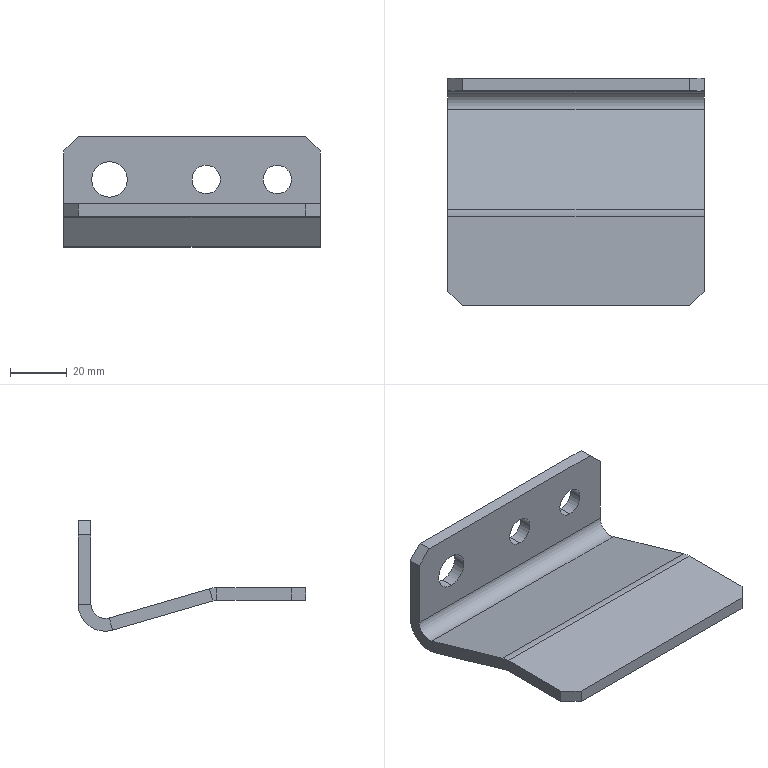Part | SolidWorks | features Chamfer 1, FlatPattern 1, ICE 1, SMBaseFlange 1, SheetMetal 1 | 1 solid | 32 faces | box 90 x 80 x 38.833 mm | volume 44176 mm3 | plane 22 | cylinder 10 | commonest cylinder face diameters 10 x6 12.5 x2 19 x2
STEP:
#1=CARTESIAN_POINT('',(75.,-4.5,-10.));
#2=VERTEX_POINT('',#1);
#3=CARTESIAN_POINT('',(75.,-4.5,-20.));
#4=VERTEX_POINT('',#3);
#5=CARTESIAN_POINT('',(75.,-4.5,-15.));
#6=DIRECTION('',(0.,-1.,0.));
#7=DIRECTION('',(0.,0.,1.));
#8=AXIS2_PLACEMENT_3D('',#5,#6,#7);
#9=CIRCLE('',#8,5.);
#10=EDGE_CURVE('',#2,#4,#9,.T.);
#11=ORIENTED_EDGE('',*,*,#10,.T.);
#12=CARTESIAN_POINT('',(75.,0.,-20.));
#13=VERTEX_POINT('',#12);
#14=CARTESIAN_POINT('',(75.,-80.001,-20.));
#15=DIRECTION('',(0.,1.,0.));
#16=VECTOR('',#15,1000.);
#17=LINE('',#14,#16);
#18=EDGE_CURVE('',#4,#13,#17,.T.);
#19=ORIENTED_EDGE('',*,*,#18,.T.);
#20=CARTESIAN_POINT('',(75.,0.,-10.));
#21=VERTEX_POINT('',#20);
#22=CARTESIAN_POINT('',(75.,0.,-15.));
#23=DIRECTION('',(0.,1.,0.));
#24=DIRECTION('',(0.,0.,1.));
#25=AXIS2_PLACEMENT_3D('',#22,#23,#24);
#26=CIRCLE('',#25,5.);
#27=EDGE_CURVE('',#13,#21,#26,.T.);
#28=ORIENTED_EDGE('',*,*,#27,.T.);
#29=CARTESIAN_POINT('',(75.,-80.001,-10.));
#30=DIRECTION('',(0.,1.,0.));
#31=VECTOR('',#30,1000.);
#32=LINE('',#29,#31);
#33=EDGE_CURVE('',#2,#21,#32,.T.);
#34=ORIENTED_EDGE('',*,*,#33,.F.);
#35=EDGE_LOOP('',(#11,#19,#28,#34));
#36=FACE_OUTER_BOUND('',#35,.T.);
#37=CARTESIAN_POINT('',(75.,-80.001,-15.));
#38=DIRECTION('',(0.,1.,0.));
#39=DIRECTION('',(0.,0.,1.));
#40=AXIS2_PLACEMENT_3D('',#37,#38,#39);
#41=CYLINDRICAL_SURFACE('',#40,5.);
#42=ADVANCED_FACE('',(#36),#41,.F.);
#43=CARTESIAN_POINT('',(50.,-4.5,-10.));
#44=VERTEX_POINT('',#43);
#45=CARTESIAN_POINT('',(50.,-4.5,-20.));
#46=VERTEX_POINT('',#45);
#47=CARTESIAN_POINT('',(50.,-4.5,-15.));
#48=DIRECTION('',(0.,-1.,0.));
#49=DIRECTION('',(0.,0.,1.));
#50=AXIS2_PLACEMENT_3D('',#47,#48,#49);
#51=CIRCLE('',#50,5.);
#52=EDGE_CURVE('',#44,#46,#51,.T.);
#53=ORIENTED_EDGE('',*,*,#52,.T.);
#54=CARTESIAN_POINT('',(50.,0.,-20.));
#55=VERTEX_POINT('',#54);
#56=CARTESIAN_POINT('',(50.,-80.001,-20.));
#57=DIRECTION('',(0.,1.,0.));
#58=VECTOR('',#57,1000.);
#59=LINE('',#56,#58);
#60=EDGE_CURVE('',#46,#55,#59,.T.);
#61=ORIENTED_EDGE('',*,*,#60,.T.);
#62=CARTESIAN_POINT('',(50.,0.,-10.));
#63=VERTEX_POINT('',#62);
#64=CARTESIAN_POINT('',(50.,0.,-15.));
#65=DIRECTION('',(0.,1.,0.));
#66=DIRECTION('',(0.,0.,1.));
#67=AXIS2_PLACEMENT_3D('',#64,#65,#66);
#68=CIRCLE('',#67,5.);
#69=EDGE_CURVE('',#55,#63,#68,.T.);
#70=ORIENTED_EDGE('',*,*,#69,.T.);
#71=CARTESIAN_POINT('',(50.,-80.001,-10.));
#72=DIRECTION('',(0.,1.,0.));
#73=VECTOR('',#72,1000.);
#74=LINE('',#71,#73);
#75=EDGE_CURVE('',#44,#63,#74,.T.);
#76=ORIENTED_EDGE('',*,*,#75,.F.);
#77=EDGE_LOOP('',(#53,#61,#70,#76));
#78=FACE_OUTER_BOUND('',#77,.T.);
#79=CARTESIAN_POINT('',(50.,-80.001,-15.));
#80=DIRECTION('',(0.,1.,0.));
#81=DIRECTION('',(0.,0.,1.));
#82=AXIS2_PLACEMENT_3D('',#79,#80,#81);
#83=CYLINDRICAL_SURFACE('',#82,5.);
#84=ADVANCED_FACE('',(#78),#83,.F.);
#85=CARTESIAN_POINT('',(16.,-4.5,-8.75));
#86=VERTEX_POINT('',#85);
#87=CARTESIAN_POINT('',(16.,-4.5,-21.25));
#88=VERTEX_POINT('',#87);
#89=CARTESIAN_POINT('',(16.,-4.5,-15.));
#90=DIRECTION('',(0.,-1.,0.));
#91=DIRECTION('',(0.,0.,1.));
#92=AXIS2_PLACEMENT_3D('',#89,#90,#91);
#93=CIRCLE('',#92,6.25);
#94=EDGE_CURVE('',#86,#88,#93,.T.);
#95=ORIENTED_EDGE('',*,*,#94,.T.);
#96=CARTESIAN_POINT('',(16.,0.,-21.25));
#97=VERTEX_POINT('',#96);
#98=CARTESIAN_POINT('',(16.,-80.001,-21.25));
#99=DIRECTION('',(0.,1.,0.));
#100=VECTOR('',#99,1000.);
#101=LINE('',#98,#100);
#102=EDGE_CURVE('',#88,#97,#101,.T.);
#103=ORIENTED_EDGE('',*,*,#102,.T.);
#104=CARTESIAN_POINT('',(16.,0.,-8.75));
#105=VERTEX_POINT('',#104);
#106=CARTESIAN_POINT('',(16.,0.,-15.));
#107=DIRECTION('',(0.,1.,0.));
#108=DIRECTION('',(0.,0.,1.));
#109=AXIS2_PLACEMENT_3D('',#106,#107,#108);
#110=CIRCLE('',#109,6.25);
#111=EDGE_CURVE('',#97,#105,#110,.T.);
#112=ORIENTED_EDGE('',*,*,#111,.T.);
#113=CARTESIAN_POINT('',(16.,-80.001,-8.75));
#114=DIRECTION('',(0.,1.,0.));
#115=VECTOR('',#114,1000.);
#116=LINE('',#113,#115);
#117=EDGE_CURVE('',#86,#105,#116,.T.);
#118=ORIENTED_EDGE('',*,*,#117,.F.);
#119=EDGE_LOOP('',(#95,#103,#112,#118));
#120=FACE_OUTER_BOUND('',#119,.T.);
#121=CARTESIAN_POINT('',(16.,-80.001,-15.));
#122=DIRECTION('',(0.,1.,0.));
#123=DIRECTION('',(0.,0.,1.));
#124=AXIS2_PLACEMENT_3D('',#121,#122,#123);
#125=CYLINDRICAL_SURFACE('',#124,6.25);
#126=ADVANCED_FACE('',(#120),#125,.F.);
#127=CARTESIAN_POINT('',(90.,-12.16,-38.453));
#128=VERTEX_POINT('',#127);
#129=CARTESIAN_POINT('',(90.,-10.9,-34.133));
#130=VERTEX_POINT('',#129);
#131=CARTESIAN_POINT('',(90.,-12.16,-38.453));
#132=DIRECTION('',(0.,0.28,0.96));
#133=VECTOR('',#132,1000.);
#134=LINE('',#131,#133);
#135=EDGE_CURVE('',#128,#130,#134,.T.);
#136=ORIENTED_EDGE('',*,*,#135,.F.);
#137=CARTESIAN_POINT('',(90.,0.,-29.333));
#138=VERTEX_POINT('',#137);
#139=CARTESIAN_POINT('',(90.,-9.5,-29.333));
#140=DIRECTION('',(-1.,0.,0.));
#141=DIRECTION('',(0.,0.,-1.));
#142=AXIS2_PLACEMENT_3D('',#139,#140,#141);
#143=CIRCLE('',#142,9.5);
#144=EDGE_CURVE('',#138,#128,#143,.T.);
#145=ORIENTED_EDGE('',*,*,#144,.F.);
#146=CARTESIAN_POINT('',(90.,-4.5,-29.333));
#147=VERTEX_POINT('',#146);
#148=CARTESIAN_POINT('',(90.,-4.5,-29.333));
#149=DIRECTION('',(0.,1.,0.));
#150=VECTOR('',#149,1000.);
#151=LINE('',#148,#150);
#152=EDGE_CURVE('',#147,#138,#151,.T.);
#153=ORIENTED_EDGE('',*,*,#152,.F.);
#154=CARTESIAN_POINT('',(90.,-9.5,-29.333));
#155=DIRECTION('',(-1.,0.,0.));
#156=DIRECTION('',(0.,0.,-1.));
#157=AXIS2_PLACEMENT_3D('',#154,#155,#156);
#158=CIRCLE('',#157,5.);
#159=EDGE_CURVE('',#147,#130,#158,.T.);
#160=ORIENTED_EDGE('',*,*,#159,.T.);
#161=EDGE_LOOP('',(#136,#145,#153,#160));
#162=FACE_OUTER_BOUND('',#161,.T.);
#163=CARTESIAN_POINT('',(90.,-12.16,-38.453));
#164=DIRECTION('',(1.,0.,0.));
#165=DIRECTION('',(0.,0.,-1.));
#166=AXIS2_PLACEMENT_3D('',#163,#164,#165);
#167=PLANE('',#166);
#168=ADVANCED_FACE('',(#162),#167,.T.);
#169=CARTESIAN_POINT('',(90.,-47.314,-28.2));
#170=VERTEX_POINT('',#169);
#171=CARTESIAN_POINT('',(90.,0.,-42.));
#172=DIRECTION('',(0.,-0.96,0.28));
#173=VECTOR('',#172,1000.);
#174=LINE('',#171,#173);
#175=EDGE_CURVE('',#128,#170,#174,.T.);
#176=ORIENTED_EDGE('',*,*,#175,.F.);
#177=ORIENTED_EDGE('',*,*,#135,.T.);
#178=CARTESIAN_POINT('',(90.,-46.054,-23.88));
#179=VERTEX_POINT('',#178);
#180=CARTESIAN_POINT('',(90.,1.26,-37.68));
#181=DIRECTION('',(0.,-0.96,0.28));
#182=VECTOR('',#181,1000.);
#183=LINE('',#180,#182);
#184=EDGE_CURVE('',#130,#179,#183,.T.);
#185=ORIENTED_EDGE('',*,*,#184,.T.);
#186=CARTESIAN_POINT('',(90.,-46.054,-23.88));
#187=DIRECTION('',(0.,-0.28,-0.96));
#188=VECTOR('',#187,1000.);
#189=LINE('',#186,#188);
#190=EDGE_CURVE('',#179,#170,#189,.T.);
#191=ORIENTED_EDGE('',*,*,#190,.T.);
#192=EDGE_LOOP('',(#176,#177,#185,#191));
#193=FACE_OUTER_BOUND('',#192,.T.);
#194=CARTESIAN_POINT('',(90.,-4.5,-29.333));
#195=DIRECTION('',(1.,0.,0.));
#196=DIRECTION('',(0.,0.,-1.));
#197=AXIS2_PLACEMENT_3D('',#194,#195,#196);
#198=PLANE('',#197);
#199=ADVANCED_FACE('',(#193),#198,.T.);
#200=CARTESIAN_POINT('',(0.,0.,-29.333));
#201=VERTEX_POINT('',#200);
#202=CARTESIAN_POINT('',(0.,-4.5,-29.333));
#203=VERTEX_POINT('',#202);
#204=CARTESIAN_POINT('',(0.,0.,-29.333));
#205=DIRECTION('',(0.,-1.,0.));
#206=VECTOR('',#205,1000.);
#207=LINE('',#204,#206);
#208=EDGE_CURVE('',#201,#203,#207,.T.);
#209=ORIENTED_EDGE('',*,*,#208,.F.);
#210=CARTESIAN_POINT('',(0.,-12.16,-38.453));
#211=VERTEX_POINT('',#210);
#212=CARTESIAN_POINT('',(0.,-9.5,-29.333));
#213=DIRECTION('',(-1.,0.,0.));
#214=DIRECTION('',(0.,0.,-1.));
#215=AXIS2_PLACEMENT_3D('',#212,#213,#214);
#216=CIRCLE('',#215,9.5);
#217=EDGE_CURVE('',#201,#211,#216,.T.);
#218=ORIENTED_EDGE('',*,*,#217,.T.);
#219=CARTESIAN_POINT('',(0.,-10.9,-34.133));
#220=VERTEX_POINT('',#219);
#221=CARTESIAN_POINT('',(0.,-10.9,-34.133));
#222=DIRECTION('',(0.,-0.28,-0.96));
#223=VECTOR('',#222,1000.);
#224=LINE('',#221,#223);
#225=EDGE_CURVE('',#220,#211,#224,.T.);
#226=ORIENTED_EDGE('',*,*,#225,.F.);
#227=CARTESIAN_POINT('',(0.,-9.5,-29.333));
#228=DIRECTION('',(-1.,0.,0.));
#229=DIRECTION('',(0.,0.,-1.));
#230=AXIS2_PLACEMENT_3D('',#227,#228,#229);
#231=CIRCLE('',#230,5.);
#232=EDGE_CURVE('',#203,#220,#231,.T.);
#233=ORIENTED_EDGE('',*,*,#232,.F.);
#234=EDGE_LOOP('',(#209,#218,#226,#233));
#235=FACE_OUTER_BOUND('',#234,.T.);
#236=CARTESIAN_POINT('',(0.,0.,-29.333));
#237=DIRECTION('',(-1.,0.,0.));
#238=DIRECTION('',(0.,0.,1.));
#239=AXIS2_PLACEMENT_3D('',#236,#237,#238);
#240=PLANE('',#239);
#241=ADVANCED_FACE('',(#235),#240,.T.);
#242=CARTESIAN_POINT('',(0.,-4.5,-5.));
#243=VERTEX_POINT('',#242);
#244=CARTESIAN_POINT('',(0.,-4.5,0.));
#245=DIRECTION('',(0.,0.,-1.));
#246=VECTOR('',#245,1000.);
#247=LINE('',#244,#246);
#248=EDGE_CURVE('',#243,#203,#247,.T.);
#249=ORIENTED_EDGE('',*,*,#248,.F.);
#250=CARTESIAN_POINT('',(0.,0.,-5.));
#251=VERTEX_POINT('',#250);
#252=CARTESIAN_POINT('',(0.,-10.9,-5.));
#253=DIRECTION('',(0.,1.,0.));
#254=VECTOR('',#253,1000.);
#255=LINE('',#252,#254);
#256=EDGE_CURVE('',#243,#251,#255,.T.);
#257=ORIENTED_EDGE('',*,*,#256,.T.);
#258=CARTESIAN_POINT('',(0.,0.,0.));
#259=DIRECTION('',(0.,0.,-1.));
#260=VECTOR('',#259,1000.);
#261=LINE('',#258,#260);
#262=EDGE_CURVE('',#251,#201,#261,.T.);
#263=ORIENTED_EDGE('',*,*,#262,.T.);
#264=ORIENTED_EDGE('',*,*,#208,.T.);
#265=EDGE_LOOP('',(#249,#257,#263,#264));
#266=FACE_OUTER_BOUND('',#265,.T.);
#267=CARTESIAN_POINT('',(0.,-10.9,-34.133));
#268=DIRECTION('',(-1.,0.,0.));
#269=DIRECTION('',(0.,0.,1.));
#270=AXIS2_PLACEMENT_3D('',#267,#268,#269);
#271=PLANE('',#270);
#272=ADVANCED_FACE('',(#266),#271,.T.);
#273=CARTESIAN_POINT('',(90.,-48.714,-28.));
#274=VERTEX_POINT('',#273);
#275=CARTESIAN_POINT('',(90.,-48.714,-23.5));
#276=VERTEX_POINT('',#275);
#277=CARTESIAN_POINT('',(90.,-48.714,-28.));
#278=DIRECTION('',(0.,0.,1.));
#279=VECTOR('',#278,1000.);
#280=LINE('',#277,#279);
#281=EDGE_CURVE('',#274,#276,#280,.T.);
#282=ORIENTED_EDGE('',*,*,#281,.F.);
#283=CARTESIAN_POINT('',(90.,-48.714,-33.));
#284=DIRECTION('',(1.,0.,0.));
#285=DIRECTION('',(0.,0.,1.));
#286=AXIS2_PLACEMENT_3D('',#283,#284,#285);
#287=CIRCLE('',#286,5.);
#288=EDGE_CURVE('',#170,#274,#287,.T.);
#289=ORIENTED_EDGE('',*,*,#288,.F.);
#290=ORIENTED_EDGE('',*,*,#190,.F.);
#291=CARTESIAN_POINT('',(90.,-48.714,-33.));
#292=DIRECTION('',(1.,0.,0.));
#293=DIRECTION('',(0.,0.,-1.));
#294=AXIS2_PLACEMENT_3D('',#291,#292,#293);
#295=CIRCLE('',#294,9.5);
#296=EDGE_CURVE('',#179,#276,#295,.T.);
#297=ORIENTED_EDGE('',*,*,#296,.T.);
#298=EDGE_LOOP('',(#282,#289,#290,#297));
#299=FACE_OUTER_BOUND('',#298,.T.);
#300=CARTESIAN_POINT('',(90.,-48.714,-28.));
#301=DIRECTION('',(1.,0.,0.));
#302=DIRECTION('',(0.,0.,-1.));
#303=AXIS2_PLACEMENT_3D('',#300,#301,#302);
#304=PLANE('',#303);
#305=ADVANCED_FACE('',(#299),#304,.T.);
#306=CARTESIAN_POINT('',(90.,-75.,-23.5));
#307=VERTEX_POINT('',#306);
#308=CARTESIAN_POINT('',(90.,-48.,-23.5));
#309=DIRECTION('',(0.,-1.,0.));
#310=VECTOR('',#309,1000.);
#311=LINE('',#308,#310);
#312=EDGE_CURVE('',#276,#307,#311,.T.);
#313=ORIENTED_EDGE('',*,*,#312,.T.);
#314=CARTESIAN_POINT('',(90.,-75.,-28.));
#315=VERTEX_POINT('',#314);
#316=CARTESIAN_POINT('',(90.,-75.,-23.88));
#317=DIRECTION('',(0.,0.,-1.));
#318=VECTOR('',#317,1000.);
#319=LINE('',#316,#318);
#320=EDGE_CURVE('',#307,#315,#319,.T.);
#321=ORIENTED_EDGE('',*,*,#320,.T.);
#322=CARTESIAN_POINT('',(90.,-48.,-28.));
#323=DIRECTION('',(0.,-1.,0.));
#324=VECTOR('',#323,1000.);
#325=LINE('',#322,#324);
#326=EDGE_CURVE('',#274,#315,#325,.T.);
#327=ORIENTED_EDGE('',*,*,#326,.F.);
#328=ORIENTED_EDGE('',*,*,#281,.T.);
#329=EDGE_LOOP('',(#313,#321,#327,#328));
#330=FACE_OUTER_BOUND('',#329,.T.);
#331=CARTESIAN_POINT('',(90.,-46.054,-23.88));
#332=DIRECTION('',(1.,0.,0.));
#333=DIRECTION('',(0.,0.,-1.));
#334=AXIS2_PLACEMENT_3D('',#331,#332,#333);
#335=PLANE('',#334);
#336=ADVANCED_FACE('',(#330),#335,.T.);
#337=CARTESIAN_POINT('',(0.,-47.314,-28.2));
#338=VERTEX_POINT('',#337);
#339=CARTESIAN_POINT('',(0.,-46.054,-23.88));
#340=VERTEX_POINT('',#339);
#341=CARTESIAN_POINT('',(0.,-47.314,-28.2));
#342=DIRECTION('',(0.,0.28,0.96));
#343=VECTOR('',#342,1000.);
#344=LINE('',#341,#343);
#345=EDGE_CURVE('',#338,#340,#344,.T.);
#346=ORIENTED_EDGE('',*,*,#345,.F.);
#347=CARTESIAN_POINT('',(0.,-48.714,-28.));
#348=VERTEX_POINT('',#347);
#349=CARTESIAN_POINT('',(0.,-48.714,-33.));
#350=DIRECTION('',(1.,0.,0.));
#351=DIRECTION('',(0.,0.,1.));
#352=AXIS2_PLACEMENT_3D('',#349,#350,#351);
#353=CIRCLE('',#352,5.);
#354=EDGE_CURVE('',#338,#348,#353,.T.);
#355=ORIENTED_EDGE('',*,*,#354,.T.);
#356=CARTESIAN_POINT('',(0.,-48.714,-23.5));
#357=VERTEX_POINT('',#356);
#358=CARTESIAN_POINT('',(0.,-48.714,-23.5));
#359=DIRECTION('',(0.,0.,-1.));
#360=VECTOR('',#359,1000.);
#361=LINE('',#358,#360);
#362=EDGE_CURVE('',#357,#348,#361,.T.);
#363=ORIENTED_EDGE('',*,*,#362,.F.);
#364=CARTESIAN_POINT('',(0.,-48.714,-33.));
#365=DIRECTION('',(1.,0.,0.));
#366=DIRECTION('',(0.,0.,-1.));
#367=AXIS2_PLACEMENT_3D('',#364,#365,#366);
#368=CIRCLE('',#367,9.5);
#369=EDGE_CURVE('',#340,#357,#368,.T.);
#370=ORIENTED_EDGE('',*,*,#369,.F.);
#371=EDGE_LOOP('',(#346,#355,#363,#370));
#372=FACE_OUTER_BOUND('',#371,.T.);
#373=CARTESIAN_POINT('',(0.,-47.314,-28.2));
#374=DIRECTION('',(-1.,0.,0.));
#375=DIRECTION('',(0.,0.,1.));
#376=AXIS2_PLACEMENT_3D('',#373,#374,#375);
#377=PLANE('',#376);
#378=ADVANCED_FACE('',(#372),#377,.T.);
#379=CARTESIAN_POINT('',(0.,0.,-42.));
#380=DIRECTION('',(0.,-0.96,0.28));
#381=VECTOR('',#380,1000.);
#382=LINE('',#379,#381);
#383=EDGE_CURVE('',#211,#338,#382,.T.);
#384=ORIENTED_EDGE('',*,*,#383,.T.);
#385=ORIENTED_EDGE('',*,*,#345,.T.);
#386=CARTESIAN_POINT('',(0.,1.26,-37.68));
#387=DIRECTION('',(0.,-0.96,0.28));
#388=VECTOR('',#387,1000.);
#389=LINE('',#386,#388);
#390=EDGE_CURVE('',#220,#340,#389,.T.);
#391=ORIENTED_EDGE('',*,*,#390,.F.);
#392=ORIENTED_EDGE('',*,*,#225,.T.);
#393=EDGE_LOOP('',(#384,#385,#391,#392));
#394=FACE_OUTER_BOUND('',#393,.T.);
#395=CARTESIAN_POINT('',(0.,-48.714,-23.5));
#396=DIRECTION('',(-1.,0.,0.));
#397=DIRECTION('',(0.,0.,1.));
#398=AXIS2_PLACEMENT_3D('',#395,#396,#397);
#399=PLANE('',#398);
#400=ADVANCED_FACE('',(#394),#399,.T.);
#401=CARTESIAN_POINT('',(0.,-75.,-23.5));
#402=VERTEX_POINT('',#401);
#403=CARTESIAN_POINT('',(0.,-48.,-23.5));
#404=DIRECTION('',(0.,-1.,0.));
#405=VECTOR('',#404,1000.);
#406=LINE('',#403,#405);
#407=EDGE_CURVE('',#357,#402,#406,.T.);
#408=ORIENTED_EDGE('',*,*,#407,.T.);
#409=CARTESIAN_POINT('',(5.,-80.,-23.5));
#410=VERTEX_POINT('',#409);
#411=CARTESIAN_POINT('',(0.,-75.,-23.5));
#412=DIRECTION('',(0.7071,-0.7071,0.));
#413=VECTOR('',#412,1000.);
#414=LINE('',#411,#413);
#415=EDGE_CURVE('',#402,#410,#414,.T.);
#416=ORIENTED_EDGE('',*,*,#415,.T.);
#417=CARTESIAN_POINT('',(85.,-80.,-23.5));
#418=VERTEX_POINT('',#417);
#419=CARTESIAN_POINT('',(90.,-80.,-23.5));
#420=DIRECTION('',(-1.,0.,0.));
#421=VECTOR('',#420,1000.);
#422=LINE('',#419,#421);
#423=EDGE_CURVE('',#418,#410,#422,.T.);
#424=ORIENTED_EDGE('',*,*,#423,.F.);
#425=CARTESIAN_POINT('',(85.,-80.,-23.5));
#426=DIRECTION('',(0.7071,0.7071,0.));
#427=VECTOR('',#426,1000.);
#428=LINE('',#425,#427);
#429=EDGE_CURVE('',#418,#307,#428,.T.);
#430=ORIENTED_EDGE('',*,*,#429,.T.);
#431=ORIENTED_EDGE('',*,*,#312,.F.);
#432=CARTESIAN_POINT('',(90.,-48.714,-23.5));
#433=DIRECTION('',(-1.,0.,0.));
#434=VECTOR('',#433,1000.);
#435=LINE('',#432,#434);
#436=EDGE_CURVE('',#276,#357,#435,.T.);
#437=ORIENTED_EDGE('',*,*,#436,.T.);
#438=EDGE_LOOP('',(#408,#416,#424,#430,#431,#437));
#439=FACE_OUTER_BOUND('',#438,.T.);
#440=CARTESIAN_POINT('',(90.,-48.,-23.5));
#441=DIRECTION('',(0.,0.,-1.));
#442=DIRECTION('',(0.,1.,0.));
#443=AXIS2_PLACEMENT_3D('',#440,#441,#442);
#444=PLANE('',#443);
#445=ADVANCED_FACE('',(#439),#444,.F.);
#446=ORIENTED_EDGE('',*,*,#423,.T.);
#447=CARTESIAN_POINT('',(5.,-80.,-28.));
#448=VERTEX_POINT('',#447);
#449=CARTESIAN_POINT('',(5.,-80.,-28.));
#450=DIRECTION('',(0.,0.,-1.));
#451=VECTOR('',#450,1000.);
#452=LINE('',#449,#451);
#453=EDGE_CURVE('',#410,#448,#452,.T.);
#454=ORIENTED_EDGE('',*,*,#453,.T.);
#455=CARTESIAN_POINT('',(85.,-80.,-28.));
#456=VERTEX_POINT('',#455);
#457=CARTESIAN_POINT('',(90.,-80.,-28.));
#458=DIRECTION('',(-1.,0.,0.));
#459=VECTOR('',#458,1000.);
#460=LINE('',#457,#459);
#461=EDGE_CURVE('',#456,#448,#460,.T.);
#462=ORIENTED_EDGE('',*,*,#461,.F.);
#463=CARTESIAN_POINT('',(85.,-80.,-28.));
#464=DIRECTION('',(0.,0.,1.));
#465=VECTOR('',#464,1000.);
#466=LINE('',#463,#465);
#467=EDGE_CURVE('',#456,#418,#466,.T.);
#468=ORIENTED_EDGE('',*,*,#467,.T.);
#469=EDGE_LOOP('',(#446,#454,#462,#468));
#470=FACE_OUTER_BOUND('',#469,.T.);
#471=CARTESIAN_POINT('',(90.,-80.,-28.));
#472=DIRECTION('',(0.,-1.,0.));
#473=DIRECTION('',(0.,0.,-1.));
#474=AXIS2_PLACEMENT_3D('',#471,#472,#473);
#475=PLANE('',#474);
#476=ADVANCED_FACE('',(#470),#475,.T.);
#477=ORIENTED_EDGE('',*,*,#461,.T.);
#478=CARTESIAN_POINT('',(0.,-75.,-28.));
#479=VERTEX_POINT('',#478);
#480=CARTESIAN_POINT('',(31.5,-106.5,-28.));
#481=DIRECTION('',(-0.7071,0.7071,0.));
#482=VECTOR('',#481,1000.);
#483=LINE('',#480,#482);
#484=EDGE_CURVE('',#448,#479,#483,.T.);
#485=ORIENTED_EDGE('',*,*,#484,.T.);
#486=CARTESIAN_POINT('',(0.,-48.,-28.));
#487=DIRECTION('',(0.,-1.,0.));
#488=VECTOR('',#487,1000.);
#489=LINE('',#486,#488);
#490=EDGE_CURVE('',#348,#479,#489,.T.);
#491=ORIENTED_EDGE('',*,*,#490,.F.);
#492=CARTESIAN_POINT('',(90.,-48.714,-28.));
#493=DIRECTION('',(-1.,0.,0.));
#494=VECTOR('',#493,1000.);
#495=LINE('',#492,#494);
#496=EDGE_CURVE('',#274,#348,#495,.T.);
#497=ORIENTED_EDGE('',*,*,#496,.F.);
#498=ORIENTED_EDGE('',*,*,#326,.T.);
#499=CARTESIAN_POINT('',(103.5,-61.5,-28.));
#500=DIRECTION('',(-0.7071,-0.7071,0.));
#501=VECTOR('',#500,1000.);
#502=LINE('',#499,#501);
#503=EDGE_CURVE('',#315,#456,#502,.T.);
#504=ORIENTED_EDGE('',*,*,#503,.T.);
#505=EDGE_LOOP('',(#477,#485,#491,#497,#498,#504));
#506=FACE_OUTER_BOUND('',#505,.T.);
#507=CARTESIAN_POINT('',(90.,-48.,-28.));
#508=DIRECTION('',(0.,0.,-1.));
#509=DIRECTION('',(0.,1.,0.));
#510=AXIS2_PLACEMENT_3D('',#507,#508,#509);
#511=PLANE('',#510);
#512=ADVANCED_FACE('',(#506),#511,.T.);
#513=ORIENTED_EDGE('',*,*,#354,.F.);
#514=CARTESIAN_POINT('',(90.,-47.314,-28.2));
#515=DIRECTION('',(-1.,0.,0.));
#516=VECTOR('',#515,1000.);
#517=LINE('',#514,#516);
#518=EDGE_CURVE('',#170,#338,#517,.T.);
#519=ORIENTED_EDGE('',*,*,#518,.F.);
#520=ORIENTED_EDGE('',*,*,#288,.T.);
#521=ORIENTED_EDGE('',*,*,#496,.T.);
#522=EDGE_LOOP('',(#513,#519,#520,#521));
#523=FACE_OUTER_BOUND('',#522,.T.);
#524=CARTESIAN_POINT('',(90.,-48.714,-33.));
#525=DIRECTION('',(-1.,0.,0.));
#526=DIRECTION('',(0.,0.,1.));
#527=AXIS2_PLACEMENT_3D('',#524,#525,#526);
#528=CYLINDRICAL_SURFACE('',#527,5.);
#529=ADVANCED_FACE('',(#523),#528,.F.);
#530=ORIENTED_EDGE('',*,*,#383,.F.);
#531=CARTESIAN_POINT('',(90.,-12.16,-38.453));
#532=DIRECTION('',(-1.,0.,0.));
#533=VECTOR('',#532,1000.);
#534=LINE('',#531,#533);
#535=EDGE_CURVE('',#128,#211,#534,.T.);
#536=ORIENTED_EDGE('',*,*,#535,.F.);
#537=ORIENTED_EDGE('',*,*,#175,.T.);
#538=ORIENTED_EDGE('',*,*,#518,.T.);
#539=EDGE_LOOP('',(#530,#536,#537,#538));
#540=FACE_OUTER_BOUND('',#539,.T.);
#541=CARTESIAN_POINT('',(90.,0.,-42.));
#542=DIRECTION('',(0.,-0.28,-0.96));
#543=DIRECTION('',(0.,0.96,-0.28));
#544=AXIS2_PLACEMENT_3D('',#541,#542,#543);
#545=PLANE('',#544);
#546=ADVANCED_FACE('',(#540),#545,.T.);
#547=ORIENTED_EDGE('',*,*,#217,.F.);
#548=CARTESIAN_POINT('',(90.,0.,-29.333));
#549=DIRECTION('',(-1.,0.,0.));
#550=VECTOR('',#549,1000.);
#551=LINE('',#548,#550);
#552=EDGE_CURVE('',#138,#201,#551,.T.);
#553=ORIENTED_EDGE('',*,*,#552,.F.);
#554=ORIENTED_EDGE('',*,*,#144,.T.);
#555=ORIENTED_EDGE('',*,*,#535,.T.);
#556=EDGE_LOOP('',(#547,#553,#554,#555));
#557=FACE_OUTER_BOUND('',#556,.T.);
#558=CARTESIAN_POINT('',(90.,-9.5,-29.333));
#559=DIRECTION('',(-1.,0.,0.));
#560=DIRECTION('',(0.,0.,1.));
#561=AXIS2_PLACEMENT_3D('',#558,#559,#560);
#562=CYLINDRICAL_SURFACE('',#561,9.5);
#563=ADVANCED_FACE('',(#557),#562,.T.);
#564=CARTESIAN_POINT('',(75.,0.,-15.));
#565=DIRECTION('',(0.,1.,0.));
#566=DIRECTION('',(0.,0.,1.));
#567=AXIS2_PLACEMENT_3D('',#564,#565,#566);
#568=CIRCLE('',#567,5.);
#569=EDGE_CURVE('',#21,#13,#568,.T.);
#570=ORIENTED_EDGE('',*,*,#569,.F.);
#571=ORIENTED_EDGE('',*,*,#27,.F.);
#572=EDGE_LOOP('',(#570,#571));
#573=FACE_BOUND('',#572,.T.);
#574=CARTESIAN_POINT('',(50.,0.,-15.));
#575=DIRECTION('',(0.,1.,0.));
#576=DIRECTION('',(0.,0.,1.));
#577=AXIS2_PLACEMENT_3D('',#574,#575,#576);
#578=CIRCLE('',#577,5.);
#579=EDGE_CURVE('',#63,#55,#578,.T.);
#580=ORIENTED_EDGE('',*,*,#579,.F.);
#581=ORIENTED_EDGE('',*,*,#69,.F.);
#582=EDGE_LOOP('',(#580,#581));
#583=FACE_BOUND('',#582,.T.);
#584=CARTESIAN_POINT('',(16.,0.,-15.));
#585=DIRECTION('',(0.,1.,0.));
#586=DIRECTION('',(0.,0.,1.));
#587=AXIS2_PLACEMENT_3D('',#584,#585,#586);
#588=CIRCLE('',#587,6.25);
#589=EDGE_CURVE('',#105,#97,#588,.T.);
#590=ORIENTED_EDGE('',*,*,#589,.F.);
#591=ORIENTED_EDGE('',*,*,#111,.F.);
#592=EDGE_LOOP('',(#590,#591));
#593=FACE_BOUND('',#592,.T.);
#594=ORIENTED_EDGE('',*,*,#262,.F.);
#595=CARTESIAN_POINT('',(5.,0.,0.));
#596=VERTEX_POINT('',#595);
#597=CARTESIAN_POINT('',(47.5,0.,42.5));
#598=DIRECTION('',(0.7071,0.,0.7071));
#599=VECTOR('',#598,1000.);
#600=LINE('',#597,#599);
#601=EDGE_CURVE('',#251,#596,#600,.T.);
#602=ORIENTED_EDGE('',*,*,#601,.T.);
#603=CARTESIAN_POINT('',(85.,0.,0.));
#604=VERTEX_POINT('',#603);
#605=CARTESIAN_POINT('',(90.,0.,0.));
#606=DIRECTION('',(-1.,0.,0.));
#607=VECTOR('',#606,1000.);
#608=LINE('',#605,#607);
#609=EDGE_CURVE('',#604,#596,#608,.T.);
#610=ORIENTED_EDGE('',*,*,#609,.F.);
#611=CARTESIAN_POINT('',(90.,0.,-5.));
#612=VERTEX_POINT('',#611);
#613=CARTESIAN_POINT('',(87.5,0.,-2.5));
#614=DIRECTION('',(0.7071,0.,-0.7071));
#615=VECTOR('',#614,1000.);
#616=LINE('',#613,#615);
#617=EDGE_CURVE('',#604,#612,#616,.T.);
#618=ORIENTED_EDGE('',*,*,#617,.T.);
#619=CARTESIAN_POINT('',(90.,0.,0.));
#620=DIRECTION('',(0.,0.,-1.));
#621=VECTOR('',#620,1000.);
#622=LINE('',#619,#621);
#623=EDGE_CURVE('',#612,#138,#622,.T.);
#624=ORIENTED_EDGE('',*,*,#623,.T.);
#625=ORIENTED_EDGE('',*,*,#552,.T.);
#626=EDGE_LOOP('',(#594,#602,#610,#618,#624,#625));
#627=FACE_OUTER_BOUND('',#626,.T.);
#628=CARTESIAN_POINT('',(90.,0.,0.));
#629=DIRECTION('',(0.,1.,0.));
#630=DIRECTION('',(0.,0.,1.));
#631=AXIS2_PLACEMENT_3D('',#628,#629,#630);
#632=PLANE('',#631);
#633=ADVANCED_FACE('',(#573,#583,#593,#627),#632,.T.);
#634=ORIENTED_EDGE('',*,*,#609,.T.);
#635=CARTESIAN_POINT('',(5.,-4.5,0.));
#636=VERTEX_POINT('',#635);
#637=CARTESIAN_POINT('',(5.,-4.5,0.));
#638=DIRECTION('',(0.,-1.,0.));
#639=VECTOR('',#638,1000.);
#640=LINE('',#637,#639);
#641=EDGE_CURVE('',#596,#636,#640,.T.);
#642=ORIENTED_EDGE('',*,*,#641,.T.);
#643=CARTESIAN_POINT('',(85.,-4.5,0.));
#644=VERTEX_POINT('',#643);
#645=CARTESIAN_POINT('',(90.,-4.5,0.));
#646=DIRECTION('',(-1.,0.,0.));
#647=VECTOR('',#646,1000.);
#648=LINE('',#645,#647);
#649=EDGE_CURVE('',#644,#636,#648,.T.);
#650=ORIENTED_EDGE('',*,*,#649,.F.);
#651=CARTESIAN_POINT('',(85.,0.,0.));
#652=DIRECTION('',(0.,1.,0.));
#653=VECTOR('',#652,1000.);
#654=LINE('',#651,#653);
#655=EDGE_CURVE('',#644,#604,#654,.T.);
#656=ORIENTED_EDGE('',*,*,#655,.T.);
#657=EDGE_LOOP('',(#634,#642,#650,#656));
#658=FACE_OUTER_BOUND('',#657,.T.);
#659=CARTESIAN_POINT('',(90.,-4.5,0.));
#660=DIRECTION('',(0.,0.,1.));
#661=DIRECTION('',(1.,0.,0.));
#662=AXIS2_PLACEMENT_3D('',#659,#660,#661);
#663=PLANE('',#662);
#664=ADVANCED_FACE('',(#658),#663,.T.);
#665=ORIENTED_EDGE('',*,*,#10,.F.);
#666=CARTESIAN_POINT('',(75.,-4.5,-15.));
#667=DIRECTION('',(0.,-1.,0.));
#668=DIRECTION('',(0.,0.,1.));
#669=AXIS2_PLACEMENT_3D('',#666,#667,#668);
#670=CIRCLE('',#669,5.);
#671=EDGE_CURVE('',#4,#2,#670,.T.);
#672=ORIENTED_EDGE('',*,*,#671,.F.);
#673=EDGE_LOOP('',(#665,#672));
#674=FACE_BOUND('',#673,.T.);
#675=ORIENTED_EDGE('',*,*,#52,.F.);
#676=CARTESIAN_POINT('',(50.,-4.5,-15.));
#677=DIRECTION('',(0.,-1.,0.));
#678=DIRECTION('',(0.,0.,1.));
#679=AXIS2_PLACEMENT_3D('',#676,#677,#678);
#680=CIRCLE('',#679,5.);
#681=EDGE_CURVE('',#46,#44,#680,.T.);
#682=ORIENTED_EDGE('',*,*,#681,.F.);
#683=EDGE_LOOP('',(#675,#682));
#684=FACE_BOUND('',#683,.T.);
#685=ORIENTED_EDGE('',*,*,#94,.F.);
#686=CARTESIAN_POINT('',(16.,-4.5,-15.));
#687=DIRECTION('',(0.,-1.,0.));
#688=DIRECTION('',(0.,0.,1.));
#689=AXIS2_PLACEMENT_3D('',#686,#687,#688);
#690=CIRCLE('',#689,6.25);
#691=EDGE_CURVE('',#88,#86,#690,.T.);
#692=ORIENTED_EDGE('',*,*,#691,.F.);
#693=EDGE_LOOP('',(#685,#692));
#694=FACE_BOUND('',#693,.T.);
#695=ORIENTED_EDGE('',*,*,#649,.T.);
#696=CARTESIAN_POINT('',(0.,-4.5,-5.));
#697=DIRECTION('',(-0.7071,0.,-0.7071));
#698=VECTOR('',#697,1000.);
#699=LINE('',#696,#698);
#700=EDGE_CURVE('',#636,#243,#699,.T.);
#701=ORIENTED_EDGE('',*,*,#700,.T.);
#702=ORIENTED_EDGE('',*,*,#248,.T.);
#703=CARTESIAN_POINT('',(90.,-4.5,-29.333));
#704=DIRECTION('',(-1.,0.,0.));
#705=VECTOR('',#704,1000.);
#706=LINE('',#703,#705);
#707=EDGE_CURVE('',#147,#203,#706,.T.);
#708=ORIENTED_EDGE('',*,*,#707,.F.);
#709=CARTESIAN_POINT('',(90.,-4.5,-5.));
#710=VERTEX_POINT('',#709);
#711=CARTESIAN_POINT('',(90.,-4.5,0.));
#712=DIRECTION('',(0.,0.,-1.));
#713=VECTOR('',#712,1000.);
#714=LINE('',#711,#713);
#715=EDGE_CURVE('',#710,#147,#714,.T.);
#716=ORIENTED_EDGE('',*,*,#715,.F.);
#717=CARTESIAN_POINT('',(85.,-4.5,0.));
#718=DIRECTION('',(-0.7071,0.,0.7071));
#719=VECTOR('',#718,1000.);
#720=LINE('',#717,#719);
#721=EDGE_CURVE('',#710,#644,#720,.T.);
#722=ORIENTED_EDGE('',*,*,#721,.T.);
#723=EDGE_LOOP('',(#695,#701,#702,#708,#716,#722));
#724=FACE_OUTER_BOUND('',#723,.T.);
#725=CARTESIAN_POINT('',(90.,-4.5,0.));
#726=DIRECTION('',(0.,1.,0.));
#727=DIRECTION('',(0.,0.,1.));
#728=AXIS2_PLACEMENT_3D('',#725,#726,#727);
#729=PLANE('',#728);
#730=ADVANCED_FACE('',(#674,#684,#694,#724),#729,.F.);
#731=ORIENTED_EDGE('',*,*,#232,.T.);
#732=CARTESIAN_POINT('',(90.,-10.9,-34.133));
#733=DIRECTION('',(-1.,0.,0.));
#734=VECTOR('',#733,1000.);
#735=LINE('',#732,#734);
#736=EDGE_CURVE('',#130,#220,#735,.T.);
#737=ORIENTED_EDGE('',*,*,#736,.F.);
#738=ORIENTED_EDGE('',*,*,#159,.F.);
#739=ORIENTED_EDGE('',*,*,#707,.T.);
#740=EDGE_LOOP('',(#731,#737,#738,#739));
#741=FACE_OUTER_BOUND('',#740,.T.);
#742=CARTESIAN_POINT('',(90.,-9.5,-29.333));
#743=DIRECTION('',(-1.,0.,0.));
#744=DIRECTION('',(0.,0.,1.));
#745=AXIS2_PLACEMENT_3D('',#742,#743,#744);
#746=CYLINDRICAL_SURFACE('',#745,5.);
#747=ADVANCED_FACE('',(#741),#746,.F.);
#748=ORIENTED_EDGE('',*,*,#390,.T.);
#749=CARTESIAN_POINT('',(90.,-46.054,-23.88));
#750=DIRECTION('',(-1.,0.,0.));
#751=VECTOR('',#750,1000.);
#752=LINE('',#749,#751);
#753=EDGE_CURVE('',#179,#340,#752,.T.);
#754=ORIENTED_EDGE('',*,*,#753,.F.);
#755=ORIENTED_EDGE('',*,*,#184,.F.);
#756=ORIENTED_EDGE('',*,*,#736,.T.);
#757=EDGE_LOOP('',(#748,#754,#755,#756));
#758=FACE_OUTER_BOUND('',#757,.T.);
#759=CARTESIAN_POINT('',(90.,1.26,-37.68));
#760=DIRECTION('',(0.,-0.28,-0.96));
#761=DIRECTION('',(0.,0.96,-0.28));
#762=AXIS2_PLACEMENT_3D('',#759,#760,#761);
#763=PLANE('',#762);
#764=ADVANCED_FACE('',(#758),#763,.F.);
#765=ORIENTED_EDGE('',*,*,#369,.T.);
#766=ORIENTED_EDGE('',*,*,#436,.F.);
#767=ORIENTED_EDGE('',*,*,#296,.F.);
#768=ORIENTED_EDGE('',*,*,#753,.T.);
#769=EDGE_LOOP('',(#765,#766,#767,#768));
#770=FACE_OUTER_BOUND('',#769,.T.);
#771=CARTESIAN_POINT('',(90.,-48.714,-33.));
#772=DIRECTION('',(-1.,0.,0.));
#773=DIRECTION('',(0.,0.,1.));
#774=AXIS2_PLACEMENT_3D('',#771,#772,#773);
#775=CYLINDRICAL_SURFACE('',#774,9.5);
#776=ADVANCED_FACE('',(#770),#775,.T.);
#777=ORIENTED_EDGE('',*,*,#623,.F.);
#778=CARTESIAN_POINT('',(90.,-4.5,-5.));
#779=DIRECTION('',(0.,-1.,0.));
#780=VECTOR('',#779,1000.);
#781=LINE('',#778,#780);
#782=EDGE_CURVE('',#612,#710,#781,.T.);
#783=ORIENTED_EDGE('',*,*,#782,.T.);
#784=ORIENTED_EDGE('',*,*,#715,.T.);
#785=ORIENTED_EDGE('',*,*,#152,.T.);
#786=EDGE_LOOP('',(#777,#783,#784,#785));
#787=FACE_OUTER_BOUND('',#786,.T.);
#788=CARTESIAN_POINT('',(90.,-48.714,-33.));
#789=DIRECTION('',(-1.,0.,0.));
#790=DIRECTION('',(0.,0.,1.));
#791=AXIS2_PLACEMENT_3D('',#788,#789,#790);
#792=PLANE('',#791);
#793=ADVANCED_FACE('',(#787),#792,.F.);
#794=ORIENTED_EDGE('',*,*,#490,.T.);
#795=CARTESIAN_POINT('',(0.,-75.,-33.));
#796=DIRECTION('',(0.,0.,1.));
#797=VECTOR('',#796,1000.);
#798=LINE('',#795,#797);
#799=EDGE_CURVE('',#479,#402,#798,.T.);
#800=ORIENTED_EDGE('',*,*,#799,.T.);
#801=ORIENTED_EDGE('',*,*,#407,.F.);
#802=ORIENTED_EDGE('',*,*,#362,.T.);
#803=EDGE_LOOP('',(#794,#800,#801,#802));
#804=FACE_OUTER_BOUND('',#803,.T.);
#805=CARTESIAN_POINT('',(0.,-48.714,-33.));
#806=DIRECTION('',(-1.,0.,0.));
#807=DIRECTION('',(0.,0.,1.));
#808=AXIS2_PLACEMENT_3D('',#805,#806,#807);
#809=PLANE('',#808);
#810=ADVANCED_FACE('',(#804),#809,.T.);
#811=ORIENTED_EDGE('',*,*,#102,.F.);
#812=ORIENTED_EDGE('',*,*,#691,.T.);
#813=ORIENTED_EDGE('',*,*,#117,.T.);
#814=ORIENTED_EDGE('',*,*,#589,.T.);
#815=EDGE_LOOP('',(#811,#812,#813,#814));
#816=FACE_OUTER_BOUND('',#815,.T.);
#817=CARTESIAN_POINT('',(16.,-80.001,-15.));
#818=DIRECTION('',(0.,1.,0.));
#819=DIRECTION('',(0.,0.,1.));
#820=AXIS2_PLACEMENT_3D('',#817,#818,#819);
#821=CYLINDRICAL_SURFACE('',#820,6.25);
#822=ADVANCED_FACE('',(#816),#821,.F.);
#823=ORIENTED_EDGE('',*,*,#60,.F.);
#824=ORIENTED_EDGE('',*,*,#681,.T.);
#825=ORIENTED_EDGE('',*,*,#75,.T.);
#826=ORIENTED_EDGE('',*,*,#579,.T.);
#827=EDGE_LOOP('',(#823,#824,#825,#826));
#828=FACE_OUTER_BOUND('',#827,.T.);
#829=CARTESIAN_POINT('',(50.,-80.001,-15.));
#830=DIRECTION('',(0.,1.,0.));
#831=DIRECTION('',(0.,0.,1.));
#832=AXIS2_PLACEMENT_3D('',#829,#830,#831);
#833=CYLINDRICAL_SURFACE('',#832,5.);
#834=ADVANCED_FACE('',(#828),#833,.F.);
#835=ORIENTED_EDGE('',*,*,#18,.F.);
#836=ORIENTED_EDGE('',*,*,#671,.T.);
#837=ORIENTED_EDGE('',*,*,#33,.T.);
#838=ORIENTED_EDGE('',*,*,#569,.T.);
#839=EDGE_LOOP('',(#835,#836,#837,#838));
#840=FACE_OUTER_BOUND('',#839,.T.);
#841=CARTESIAN_POINT('',(75.,-80.001,-15.));
#842=DIRECTION('',(0.,1.,0.));
#843=DIRECTION('',(0.,0.,1.));
#844=AXIS2_PLACEMENT_3D('',#841,#842,#843);
#845=CYLINDRICAL_SURFACE('',#844,5.);
#846=ADVANCED_FACE('',(#840),#845,.F.);
#847=ORIENTED_EDGE('',*,*,#484,.F.);
#848=ORIENTED_EDGE('',*,*,#453,.F.);
#849=ORIENTED_EDGE('',*,*,#415,.F.);
#850=ORIENTED_EDGE('',*,*,#799,.F.);
#851=EDGE_LOOP('',(#847,#848,#849,#850));
#852=FACE_OUTER_BOUND('',#851,.T.);
#853=CARTESIAN_POINT('',(0.,-75.,-33.));
#854=DIRECTION('',(0.7071,0.7071,0.));
#855=DIRECTION('',(0.,0.,1.));
#856=AXIS2_PLACEMENT_3D('',#853,#854,#855);
#857=PLANE('',#856);
#858=ADVANCED_FACE('',(#852),#857,.F.);
#859=ORIENTED_EDGE('',*,*,#503,.F.);
#860=ORIENTED_EDGE('',*,*,#320,.F.);
#861=ORIENTED_EDGE('',*,*,#429,.F.);
#862=ORIENTED_EDGE('',*,*,#467,.F.);
#863=EDGE_LOOP('',(#859,#860,#861,#862));
#864=FACE_OUTER_BOUND('',#863,.T.);
#865=CARTESIAN_POINT('',(85.,-80.,-28.));
#866=DIRECTION('',(-0.7071,0.7071,0.));
#867=DIRECTION('',(0.,0.,1.));
#868=AXIS2_PLACEMENT_3D('',#865,#866,#867);
#869=PLANE('',#868);
#870=ADVANCED_FACE('',(#864),#869,.F.);
#871=ORIENTED_EDGE('',*,*,#700,.F.);
#872=ORIENTED_EDGE('',*,*,#641,.F.);
#873=ORIENTED_EDGE('',*,*,#601,.F.);
#874=ORIENTED_EDGE('',*,*,#256,.F.);
#875=EDGE_LOOP('',(#871,#872,#873,#874));
#876=FACE_OUTER_BOUND('',#875,.T.);
#877=CARTESIAN_POINT('',(0.,-10.9,-5.));
#878=DIRECTION('',(0.7071,0.,-0.7071));
#879=DIRECTION('',(0.,1.,0.));
#880=AXIS2_PLACEMENT_3D('',#877,#878,#879);
#881=PLANE('',#880);
#882=ADVANCED_FACE('',(#876),#881,.F.);
#883=ORIENTED_EDGE('',*,*,#721,.F.);
#884=ORIENTED_EDGE('',*,*,#782,.F.);
#885=ORIENTED_EDGE('',*,*,#617,.F.);
#886=ORIENTED_EDGE('',*,*,#655,.F.);
#887=EDGE_LOOP('',(#883,#884,#885,#886));
#888=FACE_OUTER_BOUND('',#887,.T.);
#889=CARTESIAN_POINT('',(85.,-4.5,0.));
#890=DIRECTION('',(0.7071,0.,0.7071));
#891=DIRECTION('',(0.,-1.,0.));
#892=AXIS2_PLACEMENT_3D('',#889,#890,#891);
#893=PLANE('',#892);
#894=ADVANCED_FACE('',(#888),#893,.T.);
#895=CLOSED_SHELL('',(#42,#84,#126,#168,#199,#241,#272,#305,#336,#378,#400,#445,#476,#512,#529,#546,#563,#633,#664,#730,#747,#764,#776,#793,#810,#822,#834,#846,#858,#870,#882,#894));
#896=MANIFOLD_SOLID_BREP('',#895);
#897=CARTESIAN_POINT('',(0.,0.,0.));
#898=DIRECTION('',(0.,0.,1.));
#899=DIRECTION('',(1.,0.,0.));
#900=AXIS2_PLACEMENT_3D('',#897,#898,#899);
#901=(LENGTH_UNIT()NAMED_UNIT(*)SI_UNIT(.MILLI.,.METRE.));
#902=UNCERTAINTY_MEASURE_WITH_UNIT(LENGTH_MEASURE(0.00001),#901,'','');
#903=(NAMED_UNIT(*)PLANE_ANGLE_UNIT()SI_UNIT($,.RADIAN.));
#904=(NAMED_UNIT(*)SI_UNIT($,.STERADIAN.)SOLID_ANGLE_UNIT());
#905=(GEOMETRIC_REPRESENTATION_CONTEXT(3)GLOBAL_UNCERTAINTY_ASSIGNED_CONTEXT((#902))GLOBAL_UNIT_ASSIGNED_CONTEXT((#901,#903,#904))REPRESENTATION_CONTEXT('',''));
#906=ADVANCED_BREP_SHAPE_REPRESENTATION('',(#896,#900),#905);